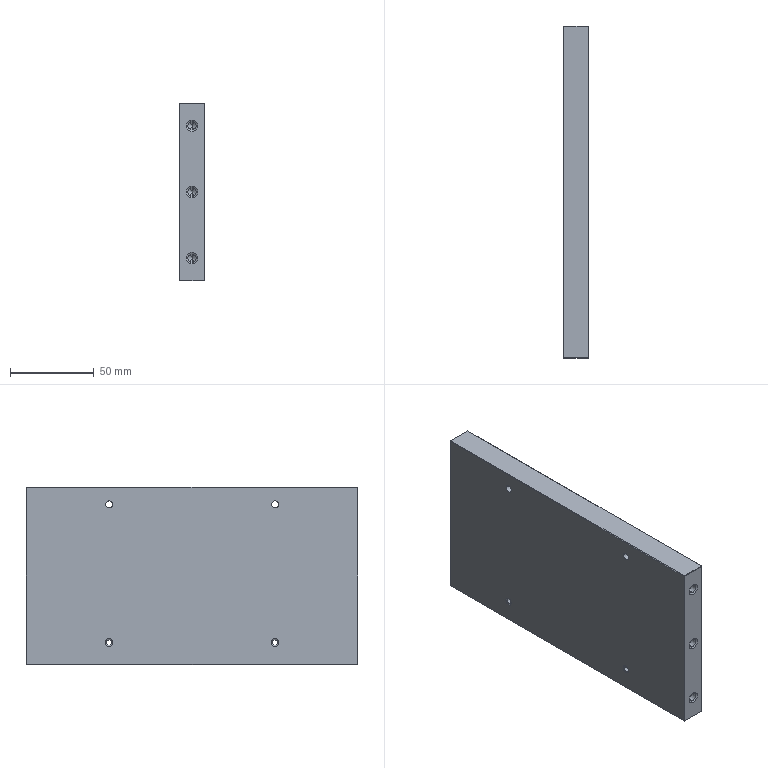Part | 1 solid | 74 faces | box 15 x 198 x 106 mm | volume 312822 mm3 | cylinder 28 | cone 28 | plane 18 | commonest cylinder face diameters 3.3 x12 5 x12 4.2 x4